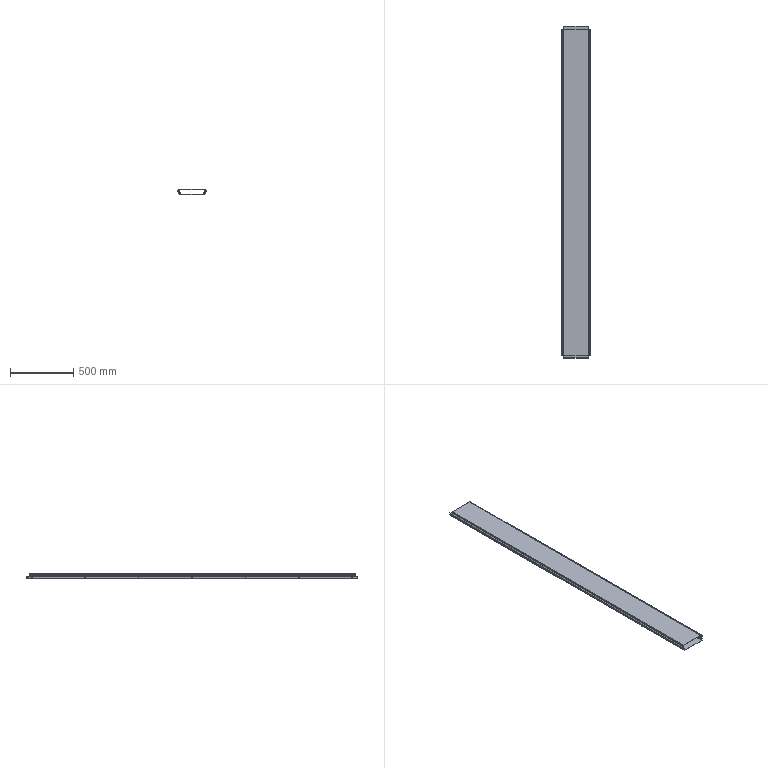Part | 18 solids | 458 faces | box 227 x 2616 x 41 mm | volume 2332302 mm3 | plane 270 | cylinder 188 | commonest cylinder face diameters 6 x28 6.2 x28 8 x28 12 x28 6.4 x24 0.6 x20